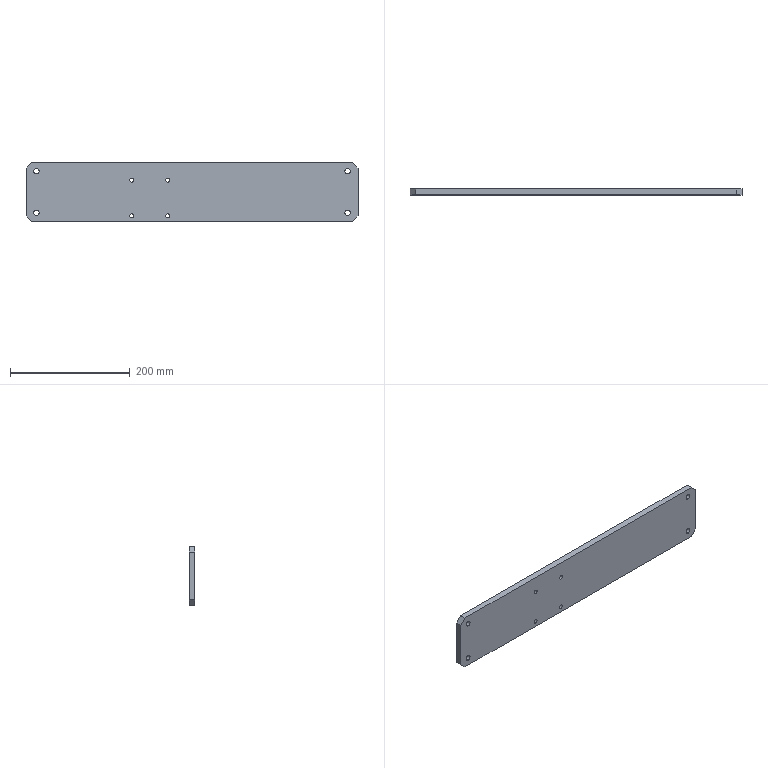Part | NX | features BREP 1 | 1 solid | 26 faces | box 555 x 10 x 100 mm | volume 549003 mm3 | cylinder 16 | plane 10 | commonest cylinder face diameters 6.8 x8 9 x8
STEP:
#1=CARTESIAN_POINT('',(-100.5,10.,16.6));
#2=VERTEX_POINT('',#1);
#3=CARTESIAN_POINT('',(-100.5,10.,23.4));
#4=VERTEX_POINT('',#3);
#5=CARTESIAN_POINT('',(-100.5,10.,20.));
#6=DIRECTION('',(0.,1.,0.));
#7=DIRECTION('',(0.,0.,1.));
#8=AXIS2_PLACEMENT_3D('',#5,#6,#7);
#9=CIRCLE('',#8,3.4);
#10=EDGE_CURVE('',#2,#4,#9,.T.);
#11=ORIENTED_EDGE('',*,*,#10,.T.);
#12=CARTESIAN_POINT('',(-100.5,0.,23.4));
#13=VERTEX_POINT('',#12);
#14=CARTESIAN_POINT('',(-100.5,0.,23.4));
#15=DIRECTION('',(0.,-1.,0.));
#16=VECTOR('',#15,1000.);
#17=LINE('',#14,#16);
#18=EDGE_CURVE('',#4,#13,#17,.T.);
#19=ORIENTED_EDGE('',*,*,#18,.T.);
#20=CARTESIAN_POINT('',(-100.5,0.,16.6));
#21=VERTEX_POINT('',#20);
#22=CARTESIAN_POINT('',(-100.5,0.,20.));
#23=DIRECTION('',(0.,-1.,0.));
#24=DIRECTION('',(0.,0.,-1.));
#25=AXIS2_PLACEMENT_3D('',#22,#23,#24);
#26=CIRCLE('',#25,3.4);
#27=EDGE_CURVE('',#13,#21,#26,.T.);
#28=ORIENTED_EDGE('',*,*,#27,.T.);
#29=CARTESIAN_POINT('',(-100.5,0.,16.6));
#30=DIRECTION('',(0.,-1.,0.));
#31=VECTOR('',#30,1000.);
#32=LINE('',#29,#31);
#33=EDGE_CURVE('',#2,#21,#32,.T.);
#34=ORIENTED_EDGE('',*,*,#33,.F.);
#35=EDGE_LOOP('',(#11,#19,#28,#34));
#36=FACE_BOUND('',#35,.T.);
#37=CARTESIAN_POINT('',(-100.5,0.,20.));
#38=DIRECTION('',(0.,-1.,0.));
#39=DIRECTION('',(0.,0.,-1.));
#40=AXIS2_PLACEMENT_3D('',#37,#38,#39);
#41=CYLINDRICAL_SURFACE('',#40,3.4);
#42=ADVANCED_FACE('',(#36),#41,.F.);
#43=CARTESIAN_POINT('',(-40.5,10.,16.6));
#44=VERTEX_POINT('',#43);
#45=CARTESIAN_POINT('',(-40.5,10.,23.4));
#46=VERTEX_POINT('',#45);
#47=CARTESIAN_POINT('',(-40.5,10.,20.));
#48=DIRECTION('',(0.,1.,0.));
#49=DIRECTION('',(0.,0.,1.));
#50=AXIS2_PLACEMENT_3D('',#47,#48,#49);
#51=CIRCLE('',#50,3.4);
#52=EDGE_CURVE('',#44,#46,#51,.T.);
#53=ORIENTED_EDGE('',*,*,#52,.T.);
#54=CARTESIAN_POINT('',(-40.5,0.,23.4));
#55=VERTEX_POINT('',#54);
#56=CARTESIAN_POINT('',(-40.5,0.,23.4));
#57=DIRECTION('',(0.,-1.,0.));
#58=VECTOR('',#57,1000.);
#59=LINE('',#56,#58);
#60=EDGE_CURVE('',#46,#55,#59,.T.);
#61=ORIENTED_EDGE('',*,*,#60,.T.);
#62=CARTESIAN_POINT('',(-40.5,0.,16.6));
#63=VERTEX_POINT('',#62);
#64=CARTESIAN_POINT('',(-40.5,0.,20.));
#65=DIRECTION('',(0.,-1.,0.));
#66=DIRECTION('',(0.,0.,-1.));
#67=AXIS2_PLACEMENT_3D('',#64,#65,#66);
#68=CIRCLE('',#67,3.4);
#69=EDGE_CURVE('',#55,#63,#68,.T.);
#70=ORIENTED_EDGE('',*,*,#69,.T.);
#71=CARTESIAN_POINT('',(-40.5,0.,16.6));
#72=DIRECTION('',(0.,-1.,0.));
#73=VECTOR('',#72,1000.);
#74=LINE('',#71,#73);
#75=EDGE_CURVE('',#44,#63,#74,.T.);
#76=ORIENTED_EDGE('',*,*,#75,.F.);
#77=EDGE_LOOP('',(#53,#61,#70,#76));
#78=FACE_BOUND('',#77,.T.);
#79=CARTESIAN_POINT('',(-40.5,0.,20.));
#80=DIRECTION('',(0.,-1.,0.));
#81=DIRECTION('',(0.,0.,-1.));
#82=AXIS2_PLACEMENT_3D('',#79,#80,#81);
#83=CYLINDRICAL_SURFACE('',#82,3.4);
#84=ADVANCED_FACE('',(#78),#83,.F.);
#85=CARTESIAN_POINT('',(-40.5,10.,-43.4));
#86=VERTEX_POINT('',#85);
#87=CARTESIAN_POINT('',(-40.5,10.,-36.6));
#88=VERTEX_POINT('',#87);
#89=CARTESIAN_POINT('',(-40.5,10.,-40.));
#90=DIRECTION('',(0.,1.,0.));
#91=DIRECTION('',(0.,0.,1.));
#92=AXIS2_PLACEMENT_3D('',#89,#90,#91);
#93=CIRCLE('',#92,3.4);
#94=EDGE_CURVE('',#86,#88,#93,.T.);
#95=ORIENTED_EDGE('',*,*,#94,.T.);
#96=CARTESIAN_POINT('',(-40.5,0.,-36.6));
#97=VERTEX_POINT('',#96);
#98=CARTESIAN_POINT('',(-40.5,0.,-36.6));
#99=DIRECTION('',(0.,-1.,0.));
#100=VECTOR('',#99,1000.);
#101=LINE('',#98,#100);
#102=EDGE_CURVE('',#88,#97,#101,.T.);
#103=ORIENTED_EDGE('',*,*,#102,.T.);
#104=CARTESIAN_POINT('',(-40.5,0.,-43.4));
#105=VERTEX_POINT('',#104);
#106=CARTESIAN_POINT('',(-40.5,0.,-40.));
#107=DIRECTION('',(0.,-1.,0.));
#108=DIRECTION('',(0.,0.,-1.));
#109=AXIS2_PLACEMENT_3D('',#106,#107,#108);
#110=CIRCLE('',#109,3.4);
#111=EDGE_CURVE('',#97,#105,#110,.T.);
#112=ORIENTED_EDGE('',*,*,#111,.T.);
#113=CARTESIAN_POINT('',(-40.5,0.,-43.4));
#114=DIRECTION('',(0.,-1.,0.));
#115=VECTOR('',#114,1000.);
#116=LINE('',#113,#115);
#117=EDGE_CURVE('',#86,#105,#116,.T.);
#118=ORIENTED_EDGE('',*,*,#117,.F.);
#119=EDGE_LOOP('',(#95,#103,#112,#118));
#120=FACE_BOUND('',#119,.T.);
#121=CARTESIAN_POINT('',(-40.5,0.,-40.));
#122=DIRECTION('',(0.,-1.,0.));
#123=DIRECTION('',(0.,0.,-1.));
#124=AXIS2_PLACEMENT_3D('',#121,#122,#123);
#125=CYLINDRICAL_SURFACE('',#124,3.4);
#126=ADVANCED_FACE('',(#120),#125,.F.);
#127=CARTESIAN_POINT('',(-100.5,10.,-43.4));
#128=VERTEX_POINT('',#127);
#129=CARTESIAN_POINT('',(-100.5,10.,-36.6));
#130=VERTEX_POINT('',#129);
#131=CARTESIAN_POINT('',(-100.5,10.,-40.));
#132=DIRECTION('',(0.,1.,0.));
#133=DIRECTION('',(0.,0.,1.));
#134=AXIS2_PLACEMENT_3D('',#131,#132,#133);
#135=CIRCLE('',#134,3.4);
#136=EDGE_CURVE('',#128,#130,#135,.T.);
#137=ORIENTED_EDGE('',*,*,#136,.T.);
#138=CARTESIAN_POINT('',(-100.5,0.,-36.6));
#139=VERTEX_POINT('',#138);
#140=CARTESIAN_POINT('',(-100.5,0.,-36.6));
#141=DIRECTION('',(0.,-1.,0.));
#142=VECTOR('',#141,1000.);
#143=LINE('',#140,#142);
#144=EDGE_CURVE('',#130,#139,#143,.T.);
#145=ORIENTED_EDGE('',*,*,#144,.T.);
#146=CARTESIAN_POINT('',(-100.5,0.,-43.4));
#147=VERTEX_POINT('',#146);
#148=CARTESIAN_POINT('',(-100.5,0.,-40.));
#149=DIRECTION('',(0.,-1.,0.));
#150=DIRECTION('',(0.,0.,-1.));
#151=AXIS2_PLACEMENT_3D('',#148,#149,#150);
#152=CIRCLE('',#151,3.4);
#153=EDGE_CURVE('',#139,#147,#152,.T.);
#154=ORIENTED_EDGE('',*,*,#153,.T.);
#155=CARTESIAN_POINT('',(-100.5,0.,-43.4));
#156=DIRECTION('',(0.,-1.,0.));
#157=VECTOR('',#156,1000.);
#158=LINE('',#155,#157);
#159=EDGE_CURVE('',#128,#147,#158,.T.);
#160=ORIENTED_EDGE('',*,*,#159,.F.);
#161=EDGE_LOOP('',(#137,#145,#154,#160));
#162=FACE_BOUND('',#161,.T.);
#163=CARTESIAN_POINT('',(-100.5,0.,-40.));
#164=DIRECTION('',(0.,-1.,0.));
#165=DIRECTION('',(0.,0.,-1.));
#166=AXIS2_PLACEMENT_3D('',#163,#164,#165);
#167=CYLINDRICAL_SURFACE('',#166,3.4);
#168=ADVANCED_FACE('',(#162),#167,.F.);
#169=CARTESIAN_POINT('',(-260.,0.,-39.5));
#170=VERTEX_POINT('',#169);
#171=CARTESIAN_POINT('',(-260.,0.,-30.5));
#172=VERTEX_POINT('',#171);
#173=CARTESIAN_POINT('',(-260.,0.,-35.));
#174=DIRECTION('',(0.,1.,0.));
#175=DIRECTION('',(0.,0.,1.));
#176=AXIS2_PLACEMENT_3D('',#173,#174,#175);
#177=CIRCLE('',#176,4.5);
#178=EDGE_CURVE('',#170,#172,#177,.T.);
#179=ORIENTED_EDGE('',*,*,#178,.F.);
#180=CARTESIAN_POINT('',(-260.,10.,-39.5));
#181=VERTEX_POINT('',#180);
#182=CARTESIAN_POINT('',(-260.,10.,-39.5));
#183=DIRECTION('',(0.,1.,0.));
#184=VECTOR('',#183,1000.);
#185=LINE('',#182,#184);
#186=EDGE_CURVE('',#181,#170,#185,.F.);
#187=ORIENTED_EDGE('',*,*,#186,.F.);
#188=CARTESIAN_POINT('',(-260.,10.,-30.5));
#189=VERTEX_POINT('',#188);
#190=CARTESIAN_POINT('',(-260.,10.,-35.));
#191=DIRECTION('',(0.,1.,0.));
#192=DIRECTION('',(0.,0.,1.));
#193=AXIS2_PLACEMENT_3D('',#190,#191,#192);
#194=CIRCLE('',#193,4.5);
#195=EDGE_CURVE('',#181,#189,#194,.T.);
#196=ORIENTED_EDGE('',*,*,#195,.T.);
#197=CARTESIAN_POINT('',(-260.,10.,-30.5));
#198=DIRECTION('',(0.,1.,0.));
#199=VECTOR('',#198,1000.);
#200=LINE('',#197,#199);
#201=EDGE_CURVE('',#189,#172,#200,.F.);
#202=ORIENTED_EDGE('',*,*,#201,.T.);
#203=EDGE_LOOP('',(#179,#187,#196,#202));
#204=FACE_BOUND('',#203,.T.);
#205=CARTESIAN_POINT('',(-260.,10.,-35.));
#206=DIRECTION('',(0.,1.,0.));
#207=DIRECTION('',(0.,0.,1.));
#208=AXIS2_PLACEMENT_3D('',#205,#206,#207);
#209=CYLINDRICAL_SURFACE('',#208,4.5);
#210=ADVANCED_FACE('',(#204),#209,.F.);
#211=CARTESIAN_POINT('',(-260.,0.,30.5));
#212=VERTEX_POINT('',#211);
#213=CARTESIAN_POINT('',(-260.,0.,39.5));
#214=VERTEX_POINT('',#213);
#215=CARTESIAN_POINT('',(-260.,0.,35.));
#216=DIRECTION('',(0.,1.,0.));
#217=DIRECTION('',(0.,0.,1.));
#218=AXIS2_PLACEMENT_3D('',#215,#216,#217);
#219=CIRCLE('',#218,4.5);
#220=EDGE_CURVE('',#212,#214,#219,.T.);
#221=ORIENTED_EDGE('',*,*,#220,.F.);
#222=CARTESIAN_POINT('',(-260.,10.,30.5));
#223=VERTEX_POINT('',#222);
#224=CARTESIAN_POINT('',(-260.,10.,30.5));
#225=DIRECTION('',(0.,1.,0.));
#226=VECTOR('',#225,1000.);
#227=LINE('',#224,#226);
#228=EDGE_CURVE('',#223,#212,#227,.F.);
#229=ORIENTED_EDGE('',*,*,#228,.F.);
#230=CARTESIAN_POINT('',(-260.,10.,39.5));
#231=VERTEX_POINT('',#230);
#232=CARTESIAN_POINT('',(-260.,10.,35.));
#233=DIRECTION('',(0.,1.,0.));
#234=DIRECTION('',(0.,0.,1.));
#235=AXIS2_PLACEMENT_3D('',#232,#233,#234);
#236=CIRCLE('',#235,4.5);
#237=EDGE_CURVE('',#223,#231,#236,.T.);
#238=ORIENTED_EDGE('',*,*,#237,.T.);
#239=CARTESIAN_POINT('',(-260.,10.,39.5));
#240=DIRECTION('',(0.,1.,0.));
#241=VECTOR('',#240,1000.);
#242=LINE('',#239,#241);
#243=EDGE_CURVE('',#231,#214,#242,.F.);
#244=ORIENTED_EDGE('',*,*,#243,.T.);
#245=EDGE_LOOP('',(#221,#229,#238,#244));
#246=FACE_BOUND('',#245,.T.);
#247=CARTESIAN_POINT('',(-260.,10.,35.));
#248=DIRECTION('',(0.,1.,0.));
#249=DIRECTION('',(0.,0.,1.));
#250=AXIS2_PLACEMENT_3D('',#247,#248,#249);
#251=CYLINDRICAL_SURFACE('',#250,4.5);
#252=ADVANCED_FACE('',(#246),#251,.F.);
#253=CARTESIAN_POINT('',(260.,0.,-39.5));
#254=VERTEX_POINT('',#253);
#255=CARTESIAN_POINT('',(260.,0.,-30.5));
#256=VERTEX_POINT('',#255);
#257=CARTESIAN_POINT('',(260.,0.,-35.));
#258=DIRECTION('',(0.,1.,0.));
#259=DIRECTION('',(0.,0.,1.));
#260=AXIS2_PLACEMENT_3D('',#257,#258,#259);
#261=CIRCLE('',#260,4.5);
#262=EDGE_CURVE('',#254,#256,#261,.T.);
#263=ORIENTED_EDGE('',*,*,#262,.F.);
#264=CARTESIAN_POINT('',(260.,10.,-39.5));
#265=VERTEX_POINT('',#264);
#266=CARTESIAN_POINT('',(260.,10.,-39.5));
#267=DIRECTION('',(0.,1.,0.));
#268=VECTOR('',#267,1000.);
#269=LINE('',#266,#268);
#270=EDGE_CURVE('',#265,#254,#269,.F.);
#271=ORIENTED_EDGE('',*,*,#270,.F.);
#272=CARTESIAN_POINT('',(260.,10.,-30.5));
#273=VERTEX_POINT('',#272);
#274=CARTESIAN_POINT('',(260.,10.,-35.));
#275=DIRECTION('',(0.,1.,0.));
#276=DIRECTION('',(0.,0.,1.));
#277=AXIS2_PLACEMENT_3D('',#274,#275,#276);
#278=CIRCLE('',#277,4.5);
#279=EDGE_CURVE('',#265,#273,#278,.T.);
#280=ORIENTED_EDGE('',*,*,#279,.T.);
#281=CARTESIAN_POINT('',(260.,10.,-30.5));
#282=DIRECTION('',(0.,1.,0.));
#283=VECTOR('',#282,1000.);
#284=LINE('',#281,#283);
#285=EDGE_CURVE('',#273,#256,#284,.F.);
#286=ORIENTED_EDGE('',*,*,#285,.T.);
#287=EDGE_LOOP('',(#263,#271,#280,#286));
#288=FACE_BOUND('',#287,.T.);
#289=CARTESIAN_POINT('',(260.,10.,-35.));
#290=DIRECTION('',(0.,1.,0.));
#291=DIRECTION('',(0.,0.,1.));
#292=AXIS2_PLACEMENT_3D('',#289,#290,#291);
#293=CYLINDRICAL_SURFACE('',#292,4.5);
#294=ADVANCED_FACE('',(#288),#293,.F.);
#295=CARTESIAN_POINT('',(260.,0.,30.5));
#296=VERTEX_POINT('',#295);
#297=CARTESIAN_POINT('',(260.,0.,39.5));
#298=VERTEX_POINT('',#297);
#299=CARTESIAN_POINT('',(260.,0.,35.));
#300=DIRECTION('',(0.,1.,0.));
#301=DIRECTION('',(0.,0.,1.));
#302=AXIS2_PLACEMENT_3D('',#299,#300,#301);
#303=CIRCLE('',#302,4.5);
#304=EDGE_CURVE('',#296,#298,#303,.T.);
#305=ORIENTED_EDGE('',*,*,#304,.F.);
#306=CARTESIAN_POINT('',(260.,10.,30.5));
#307=VERTEX_POINT('',#306);
#308=CARTESIAN_POINT('',(260.,10.,30.5));
#309=DIRECTION('',(0.,1.,0.));
#310=VECTOR('',#309,1000.);
#311=LINE('',#308,#310);
#312=EDGE_CURVE('',#307,#296,#311,.F.);
#313=ORIENTED_EDGE('',*,*,#312,.F.);
#314=CARTESIAN_POINT('',(260.,10.,39.5));
#315=VERTEX_POINT('',#314);
#316=CARTESIAN_POINT('',(260.,10.,35.));
#317=DIRECTION('',(0.,1.,0.));
#318=DIRECTION('',(0.,0.,1.));
#319=AXIS2_PLACEMENT_3D('',#316,#317,#318);
#320=CIRCLE('',#319,4.5);
#321=EDGE_CURVE('',#307,#315,#320,.T.);
#322=ORIENTED_EDGE('',*,*,#321,.T.);
#323=CARTESIAN_POINT('',(260.,10.,39.5));
#324=DIRECTION('',(0.,1.,0.));
#325=VECTOR('',#324,1000.);
#326=LINE('',#323,#325);
#327=EDGE_CURVE('',#315,#298,#326,.F.);
#328=ORIENTED_EDGE('',*,*,#327,.T.);
#329=EDGE_LOOP('',(#305,#313,#322,#328));
#330=FACE_BOUND('',#329,.T.);
#331=CARTESIAN_POINT('',(260.,10.,35.));
#332=DIRECTION('',(0.,1.,0.));
#333=DIRECTION('',(0.,0.,1.));
#334=AXIS2_PLACEMENT_3D('',#331,#332,#333);
#335=CYLINDRICAL_SURFACE('',#334,4.5);
#336=ADVANCED_FACE('',(#330),#335,.F.);
#337=CARTESIAN_POINT('',(277.5,10.,40.));
#338=VERTEX_POINT('',#337);
#339=CARTESIAN_POINT('',(277.5,10.,-40.));
#340=VERTEX_POINT('',#339);
#341=CARTESIAN_POINT('',(277.5,10.,-50.));
#342=DIRECTION('',(0.,0.,-1.));
#343=VECTOR('',#342,1000.);
#344=LINE('',#341,#343);
#345=EDGE_CURVE('',#338,#340,#344,.T.);
#346=ORIENTED_EDGE('',*,*,#345,.F.);
#347=CARTESIAN_POINT('',(277.5,0.,40.));
#348=VERTEX_POINT('',#347);
#349=CARTESIAN_POINT('',(277.5,10.,40.));
#350=DIRECTION('',(0.,-1.,0.));
#351=VECTOR('',#350,1000.);
#352=LINE('',#349,#351);
#353=EDGE_CURVE('',#338,#348,#352,.T.);
#354=ORIENTED_EDGE('',*,*,#353,.T.);
#355=CARTESIAN_POINT('',(277.5,0.,-40.));
#356=VERTEX_POINT('',#355);
#357=CARTESIAN_POINT('',(277.5,0.,-50.));
#358=DIRECTION('',(0.,0.,-1.));
#359=VECTOR('',#358,1000.);
#360=LINE('',#357,#359);
#361=EDGE_CURVE('',#348,#356,#360,.T.);
#362=ORIENTED_EDGE('',*,*,#361,.T.);
#363=CARTESIAN_POINT('',(277.5,10.,-40.));
#364=DIRECTION('',(0.,1.,0.));
#365=VECTOR('',#364,1000.);
#366=LINE('',#363,#365);
#367=EDGE_CURVE('',#356,#340,#366,.T.);
#368=ORIENTED_EDGE('',*,*,#367,.T.);
#369=EDGE_LOOP('',(#346,#354,#362,#368));
#370=FACE_BOUND('',#369,.T.);
#371=CARTESIAN_POINT('',(277.5,10.,-50.));
#372=DIRECTION('',(-1.,0.,0.));
#373=DIRECTION('',(0.,1.,0.));
#374=AXIS2_PLACEMENT_3D('',#371,#372,#373);
#375=PLANE('',#374);
#376=ADVANCED_FACE('',(#370),#375,.F.);
#377=CARTESIAN_POINT('',(267.5,10.,-50.));
#378=VERTEX_POINT('',#377);
#379=CARTESIAN_POINT('',(-267.5,10.,-50.));
#380=VERTEX_POINT('',#379);
#381=CARTESIAN_POINT('',(-277.5,10.,-50.));
#382=DIRECTION('',(-1.,0.,0.));
#383=VECTOR('',#382,1000.);
#384=LINE('',#381,#383);
#385=EDGE_CURVE('',#378,#380,#384,.T.);
#386=ORIENTED_EDGE('',*,*,#385,.F.);
#387=CARTESIAN_POINT('',(267.5,0.,-50.));
#388=VERTEX_POINT('',#387);
#389=CARTESIAN_POINT('',(267.5,10.,-50.));
#390=DIRECTION('',(0.,-1.,0.));
#391=VECTOR('',#390,1000.);
#392=LINE('',#389,#391);
#393=EDGE_CURVE('',#378,#388,#392,.T.);
#394=ORIENTED_EDGE('',*,*,#393,.T.);
#395=CARTESIAN_POINT('',(-267.5,0.,-50.));
#396=VERTEX_POINT('',#395);
#397=CARTESIAN_POINT('',(-277.5,0.,-50.));
#398=DIRECTION('',(-1.,0.,0.));
#399=VECTOR('',#398,1000.);
#400=LINE('',#397,#399);
#401=EDGE_CURVE('',#388,#396,#400,.T.);
#402=ORIENTED_EDGE('',*,*,#401,.T.);
#403=CARTESIAN_POINT('',(-267.5,10.,-50.));
#404=DIRECTION('',(0.,1.,0.));
#405=VECTOR('',#404,1000.);
#406=LINE('',#403,#405);
#407=EDGE_CURVE('',#396,#380,#406,.T.);
#408=ORIENTED_EDGE('',*,*,#407,.T.);
#409=EDGE_LOOP('',(#386,#394,#402,#408));
#410=FACE_BOUND('',#409,.T.);
#411=CARTESIAN_POINT('',(-277.5,10.,-50.));
#412=DIRECTION('',(0.,0.,1.));
#413=DIRECTION('',(1.,0.,0.));
#414=AXIS2_PLACEMENT_3D('',#411,#412,#413);
#415=PLANE('',#414);
#416=ADVANCED_FACE('',(#410),#415,.F.);
#417=CARTESIAN_POINT('',(-277.5,0.,-40.));
#418=VERTEX_POINT('',#417);
#419=CARTESIAN_POINT('',(-277.5,0.,40.));
#420=VERTEX_POINT('',#419);
#421=CARTESIAN_POINT('',(-277.5,0.,-50.));
#422=DIRECTION('',(0.,0.,1.));
#423=VECTOR('',#422,1000.);
#424=LINE('',#421,#423);
#425=EDGE_CURVE('',#418,#420,#424,.T.);
#426=ORIENTED_EDGE('',*,*,#425,.T.);
#427=CARTESIAN_POINT('',(-277.5,10.,40.));
#428=VERTEX_POINT('',#427);
#429=CARTESIAN_POINT('',(-277.5,10.,40.));
#430=DIRECTION('',(0.,1.,0.));
#431=VECTOR('',#430,1000.);
#432=LINE('',#429,#431);
#433=EDGE_CURVE('',#420,#428,#432,.T.);
#434=ORIENTED_EDGE('',*,*,#433,.T.);
#435=CARTESIAN_POINT('',(-277.5,10.,-40.));
#436=VERTEX_POINT('',#435);
#437=CARTESIAN_POINT('',(-277.5,10.,-50.));
#438=DIRECTION('',(0.,0.,1.));
#439=VECTOR('',#438,1000.);
#440=LINE('',#437,#439);
#441=EDGE_CURVE('',#436,#428,#440,.T.);
#442=ORIENTED_EDGE('',*,*,#441,.F.);
#443=CARTESIAN_POINT('',(-277.5,10.,-40.));
#444=DIRECTION('',(0.,-1.,0.));
#445=VECTOR('',#444,1000.);
#446=LINE('',#443,#445);
#447=EDGE_CURVE('',#436,#418,#446,.T.);
#448=ORIENTED_EDGE('',*,*,#447,.T.);
#449=EDGE_LOOP('',(#426,#434,#442,#448));
#450=FACE_BOUND('',#449,.T.);
#451=CARTESIAN_POINT('',(-277.5,10.,-50.));
#452=DIRECTION('',(1.,0.,0.));
#453=DIRECTION('',(0.,0.,-1.));
#454=AXIS2_PLACEMENT_3D('',#451,#452,#453);
#455=PLANE('',#454);
#456=ADVANCED_FACE('',(#450),#455,.F.);
#457=CARTESIAN_POINT('',(-267.5,0.,50.));
#458=VERTEX_POINT('',#457);
#459=CARTESIAN_POINT('',(267.5,0.,50.));
#460=VERTEX_POINT('',#459);
#461=CARTESIAN_POINT('',(-277.5,0.,50.));
#462=DIRECTION('',(1.,0.,0.));
#463=VECTOR('',#462,1000.);
#464=LINE('',#461,#463);
#465=EDGE_CURVE('',#458,#460,#464,.T.);
#466=ORIENTED_EDGE('',*,*,#465,.T.);
#467=CARTESIAN_POINT('',(267.5,10.,50.));
#468=VERTEX_POINT('',#467);
#469=CARTESIAN_POINT('',(267.5,10.,50.));
#470=DIRECTION('',(0.,1.,0.));
#471=VECTOR('',#470,1000.);
#472=LINE('',#469,#471);
#473=EDGE_CURVE('',#460,#468,#472,.T.);
#474=ORIENTED_EDGE('',*,*,#473,.T.);
#475=CARTESIAN_POINT('',(-267.5,10.,50.));
#476=VERTEX_POINT('',#475);
#477=CARTESIAN_POINT('',(-277.5,10.,50.));
#478=DIRECTION('',(1.,0.,0.));
#479=VECTOR('',#478,1000.);
#480=LINE('',#477,#479);
#481=EDGE_CURVE('',#476,#468,#480,.T.);
#482=ORIENTED_EDGE('',*,*,#481,.F.);
#483=CARTESIAN_POINT('',(-267.5,10.,50.));
#484=DIRECTION('',(0.,-1.,0.));
#485=VECTOR('',#484,1000.);
#486=LINE('',#483,#485);
#487=EDGE_CURVE('',#476,#458,#486,.T.);
#488=ORIENTED_EDGE('',*,*,#487,.T.);
#489=EDGE_LOOP('',(#466,#474,#482,#488));
#490=FACE_BOUND('',#489,.T.);
#491=CARTESIAN_POINT('',(-277.5,10.,50.));
#492=DIRECTION('',(0.,0.,-1.));
#493=DIRECTION('',(0.,-1.,0.));
#494=AXIS2_PLACEMENT_3D('',#491,#492,#493);
#495=PLANE('',#494);
#496=ADVANCED_FACE('',(#490),#495,.F.);
#497=ORIENTED_EDGE('',*,*,#481,.T.);
#498=CARTESIAN_POINT('',(158.75,10.,158.75));
#499=DIRECTION('',(0.7071,0.,-0.7071));
#500=VECTOR('',#499,1000.);
#501=LINE('',#498,#500);
#502=EDGE_CURVE('',#468,#338,#501,.T.);
#503=ORIENTED_EDGE('',*,*,#502,.T.);
#504=ORIENTED_EDGE('',*,*,#345,.T.);
#505=CARTESIAN_POINT('',(158.75,10.,-158.75));
#506=DIRECTION('',(-0.7071,0.,-0.7071));
#507=VECTOR('',#506,1000.);
#508=LINE('',#505,#507);
#509=EDGE_CURVE('',#340,#378,#508,.T.);
#510=ORIENTED_EDGE('',*,*,#509,.T.);
#511=ORIENTED_EDGE('',*,*,#385,.T.);
#512=CARTESIAN_POINT('',(-158.75,10.,-158.75));
#513=DIRECTION('',(-0.7071,0.,0.7071));
#514=VECTOR('',#513,1000.);
#515=LINE('',#512,#514);
#516=EDGE_CURVE('',#380,#436,#515,.T.);
#517=ORIENTED_EDGE('',*,*,#516,.T.);
#518=ORIENTED_EDGE('',*,*,#441,.T.);
#519=CARTESIAN_POINT('',(-158.75,10.,158.75));
#520=DIRECTION('',(0.7071,0.,0.7071));
#521=VECTOR('',#520,1000.);
#522=LINE('',#519,#521);
#523=EDGE_CURVE('',#428,#476,#522,.T.);
#524=ORIENTED_EDGE('',*,*,#523,.T.);
#525=EDGE_LOOP('',(#497,#503,#504,#510,#511,#517,#518,#524));
#526=FACE_BOUND('',#525,.T.);
#527=ORIENTED_EDGE('',*,*,#10,.F.);
#528=CARTESIAN_POINT('',(-100.5,10.,20.));
#529=DIRECTION('',(0.,1.,0.));
#530=DIRECTION('',(0.,0.,1.));
#531=AXIS2_PLACEMENT_3D('',#528,#529,#530);
#532=CIRCLE('',#531,3.4);
#533=EDGE_CURVE('',#4,#2,#532,.T.);
#534=ORIENTED_EDGE('',*,*,#533,.F.);
#535=EDGE_LOOP('',(#527,#534));
#536=FACE_BOUND('',#535,.T.);
#537=ORIENTED_EDGE('',*,*,#52,.F.);
#538=CARTESIAN_POINT('',(-40.5,10.,20.));
#539=DIRECTION('',(0.,1.,0.));
#540=DIRECTION('',(0.,0.,1.));
#541=AXIS2_PLACEMENT_3D('',#538,#539,#540);
#542=CIRCLE('',#541,3.4);
#543=EDGE_CURVE('',#46,#44,#542,.T.);
#544=ORIENTED_EDGE('',*,*,#543,.F.);
#545=EDGE_LOOP('',(#537,#544));
#546=FACE_BOUND('',#545,.T.);
#547=ORIENTED_EDGE('',*,*,#94,.F.);
#548=CARTESIAN_POINT('',(-40.5,10.,-40.));
#549=DIRECTION('',(0.,1.,0.));
#550=DIRECTION('',(0.,0.,1.));
#551=AXIS2_PLACEMENT_3D('',#548,#549,#550);
#552=CIRCLE('',#551,3.4);
#553=EDGE_CURVE('',#88,#86,#552,.T.);
#554=ORIENTED_EDGE('',*,*,#553,.F.);
#555=EDGE_LOOP('',(#547,#554));
#556=FACE_BOUND('',#555,.T.);
#557=ORIENTED_EDGE('',*,*,#136,.F.);
#558=CARTESIAN_POINT('',(-100.5,10.,-40.));
#559=DIRECTION('',(0.,1.,0.));
#560=DIRECTION('',(0.,0.,1.));
#561=AXIS2_PLACEMENT_3D('',#558,#559,#560);
#562=CIRCLE('',#561,3.4);
#563=EDGE_CURVE('',#130,#128,#562,.T.);
#564=ORIENTED_EDGE('',*,*,#563,.F.);
#565=EDGE_LOOP('',(#557,#564));
#566=FACE_BOUND('',#565,.T.);
#567=CARTESIAN_POINT('',(-260.,10.,-35.));
#568=DIRECTION('',(0.,1.,0.));
#569=DIRECTION('',(0.,0.,1.));
#570=AXIS2_PLACEMENT_3D('',#567,#568,#569);
#571=CIRCLE('',#570,4.5);
#572=EDGE_CURVE('',#189,#181,#571,.T.);
#573=ORIENTED_EDGE('',*,*,#572,.F.);
#574=ORIENTED_EDGE('',*,*,#195,.F.);
#575=EDGE_LOOP('',(#573,#574));
#576=FACE_BOUND('',#575,.T.);
#577=CARTESIAN_POINT('',(-260.,10.,35.));
#578=DIRECTION('',(0.,1.,0.));
#579=DIRECTION('',(0.,0.,1.));
#580=AXIS2_PLACEMENT_3D('',#577,#578,#579);
#581=CIRCLE('',#580,4.5);
#582=EDGE_CURVE('',#231,#223,#581,.T.);
#583=ORIENTED_EDGE('',*,*,#582,.F.);
#584=ORIENTED_EDGE('',*,*,#237,.F.);
#585=EDGE_LOOP('',(#583,#584));
#586=FACE_BOUND('',#585,.T.);
#587=CARTESIAN_POINT('',(260.,10.,-35.));
#588=DIRECTION('',(0.,1.,0.));
#589=DIRECTION('',(0.,0.,1.));
#590=AXIS2_PLACEMENT_3D('',#587,#588,#589);
#591=CIRCLE('',#590,4.5);
#592=EDGE_CURVE('',#273,#265,#591,.T.);
#593=ORIENTED_EDGE('',*,*,#592,.F.);
#594=ORIENTED_EDGE('',*,*,#279,.F.);
#595=EDGE_LOOP('',(#593,#594));
#596=FACE_BOUND('',#595,.T.);
#597=CARTESIAN_POINT('',(260.,10.,35.));
#598=DIRECTION('',(0.,1.,0.));
#599=DIRECTION('',(0.,0.,1.));
#600=AXIS2_PLACEMENT_3D('',#597,#598,#599);
#601=CIRCLE('',#600,4.5);
#602=EDGE_CURVE('',#315,#307,#601,.T.);
#603=ORIENTED_EDGE('',*,*,#602,.F.);
#604=ORIENTED_EDGE('',*,*,#321,.F.);
#605=EDGE_LOOP('',(#603,#604));
#606=FACE_BOUND('',#605,.T.);
#607=CARTESIAN_POINT('',(0.,10.,0.));
#608=DIRECTION('',(0.,1.,0.));
#609=DIRECTION('',(1.,0.,0.));
#610=AXIS2_PLACEMENT_3D('',#607,#608,#609);
#611=PLANE('',#610);
#612=ADVANCED_FACE('',(#526,#536,#546,#556,#566,#576,#586,#596,#606),#611,.T.);
#613=ORIENTED_EDGE('',*,*,#361,.F.);
#614=CARTESIAN_POINT('',(277.5,0.,40.));
#615=DIRECTION('',(-0.7071,0.,0.7071));
#616=VECTOR('',#615,1000.);
#617=LINE('',#614,#616);
#618=EDGE_CURVE('',#348,#460,#617,.T.);
#619=ORIENTED_EDGE('',*,*,#618,.T.);
#620=ORIENTED_EDGE('',*,*,#465,.F.);
#621=CARTESIAN_POINT('',(-267.5,0.,50.));
#622=DIRECTION('',(-0.7071,0.,-0.7071));
#623=VECTOR('',#622,1000.);
#624=LINE('',#621,#623);
#625=EDGE_CURVE('',#458,#420,#624,.T.);
#626=ORIENTED_EDGE('',*,*,#625,.T.);
#627=ORIENTED_EDGE('',*,*,#425,.F.);
#628=CARTESIAN_POINT('',(-277.5,0.,-40.));
#629=DIRECTION('',(0.7071,0.,-0.7071));
#630=VECTOR('',#629,1000.);
#631=LINE('',#628,#630);
#632=EDGE_CURVE('',#418,#396,#631,.T.);
#633=ORIENTED_EDGE('',*,*,#632,.T.);
#634=ORIENTED_EDGE('',*,*,#401,.F.);
#635=CARTESIAN_POINT('',(267.5,0.,-50.));
#636=DIRECTION('',(0.7071,0.,0.7071));
#637=VECTOR('',#636,1000.);
#638=LINE('',#635,#637);
#639=EDGE_CURVE('',#388,#356,#638,.T.);
#640=ORIENTED_EDGE('',*,*,#639,.T.);
#641=EDGE_LOOP('',(#613,#619,#620,#626,#627,#633,#634,#640));
#642=FACE_BOUND('',#641,.T.);
#643=CARTESIAN_POINT('',(-100.5,0.,20.));
#644=DIRECTION('',(0.,-1.,0.));
#645=DIRECTION('',(0.,0.,-1.));
#646=AXIS2_PLACEMENT_3D('',#643,#644,#645);
#647=CIRCLE('',#646,3.4);
#648=EDGE_CURVE('',#21,#13,#647,.T.);
#649=ORIENTED_EDGE('',*,*,#648,.F.);
#650=ORIENTED_EDGE('',*,*,#27,.F.);
#651=EDGE_LOOP('',(#649,#650));
#652=FACE_BOUND('',#651,.T.);
#653=CARTESIAN_POINT('',(-40.5,0.,20.));
#654=DIRECTION('',(0.,-1.,0.));
#655=DIRECTION('',(0.,0.,-1.));
#656=AXIS2_PLACEMENT_3D('',#653,#654,#655);
#657=CIRCLE('',#656,3.4);
#658=EDGE_CURVE('',#63,#55,#657,.T.);
#659=ORIENTED_EDGE('',*,*,#658,.F.);
#660=ORIENTED_EDGE('',*,*,#69,.F.);
#661=EDGE_LOOP('',(#659,#660));
#662=FACE_BOUND('',#661,.T.);
#663=CARTESIAN_POINT('',(-40.5,0.,-40.));
#664=DIRECTION('',(0.,-1.,0.));
#665=DIRECTION('',(0.,0.,-1.));
#666=AXIS2_PLACEMENT_3D('',#663,#664,#665);
#667=CIRCLE('',#666,3.4);
#668=EDGE_CURVE('',#105,#97,#667,.T.);
#669=ORIENTED_EDGE('',*,*,#668,.F.);
#670=ORIENTED_EDGE('',*,*,#111,.F.);
#671=EDGE_LOOP('',(#669,#670));
#672=FACE_BOUND('',#671,.T.);
#673=CARTESIAN_POINT('',(-100.5,0.,-40.));
#674=DIRECTION('',(0.,-1.,0.));
#675=DIRECTION('',(0.,0.,-1.));
#676=AXIS2_PLACEMENT_3D('',#673,#674,#675);
#677=CIRCLE('',#676,3.4);
#678=EDGE_CURVE('',#147,#139,#677,.T.);
#679=ORIENTED_EDGE('',*,*,#678,.F.);
#680=ORIENTED_EDGE('',*,*,#153,.F.);
#681=EDGE_LOOP('',(#679,#680));
#682=FACE_BOUND('',#681,.T.);
#683=CARTESIAN_POINT('',(-260.,0.,-35.));
#684=DIRECTION('',(0.,1.,0.));
#685=DIRECTION('',(0.,0.,1.));
#686=AXIS2_PLACEMENT_3D('',#683,#684,#685);
#687=CIRCLE('',#686,4.5);
#688=EDGE_CURVE('',#172,#170,#687,.T.);
#689=ORIENTED_EDGE('',*,*,#688,.T.);
#690=ORIENTED_EDGE('',*,*,#178,.T.);
#691=EDGE_LOOP('',(#689,#690));
#692=FACE_BOUND('',#691,.T.);
#693=CARTESIAN_POINT('',(-260.,0.,35.));
#694=DIRECTION('',(0.,1.,0.));
#695=DIRECTION('',(0.,0.,1.));
#696=AXIS2_PLACEMENT_3D('',#693,#694,#695);
#697=CIRCLE('',#696,4.5);
#698=EDGE_CURVE('',#214,#212,#697,.T.);
#699=ORIENTED_EDGE('',*,*,#698,.T.);
#700=ORIENTED_EDGE('',*,*,#220,.T.);
#701=EDGE_LOOP('',(#699,#700));
#702=FACE_BOUND('',#701,.T.);
#703=CARTESIAN_POINT('',(260.,0.,-35.));
#704=DIRECTION('',(0.,1.,0.));
#705=DIRECTION('',(0.,0.,1.));
#706=AXIS2_PLACEMENT_3D('',#703,#704,#705);
#707=CIRCLE('',#706,4.5);
#708=EDGE_CURVE('',#256,#254,#707,.T.);
#709=ORIENTED_EDGE('',*,*,#708,.T.);
#710=ORIENTED_EDGE('',*,*,#262,.T.);
#711=EDGE_LOOP('',(#709,#710));
#712=FACE_BOUND('',#711,.T.);
#713=CARTESIAN_POINT('',(260.,0.,35.));
#714=DIRECTION('',(0.,1.,0.));
#715=DIRECTION('',(0.,0.,1.));
#716=AXIS2_PLACEMENT_3D('',#713,#714,#715);
#717=CIRCLE('',#716,4.5);
#718=EDGE_CURVE('',#298,#296,#717,.T.);
#719=ORIENTED_EDGE('',*,*,#718,.T.);
#720=ORIENTED_EDGE('',*,*,#304,.T.);
#721=EDGE_LOOP('',(#719,#720));
#722=FACE_BOUND('',#721,.T.);
#723=CARTESIAN_POINT('',(0.,0.,0.));
#724=DIRECTION('',(0.,1.,0.));
#725=DIRECTION('',(1.,0.,0.));
#726=AXIS2_PLACEMENT_3D('',#723,#724,#725);
#727=PLANE('',#726);
#728=ADVANCED_FACE('',(#642,#652,#662,#672,#682,#692,#702,#712,#722),#727,.F.);
#729=ORIENTED_EDGE('',*,*,#312,.T.);
#730=ORIENTED_EDGE('',*,*,#718,.F.);
#731=ORIENTED_EDGE('',*,*,#327,.F.);
#732=ORIENTED_EDGE('',*,*,#602,.T.);
#733=EDGE_LOOP('',(#729,#730,#731,#732));
#734=FACE_BOUND('',#733,.T.);
#735=CARTESIAN_POINT('',(260.,10.,35.));
#736=DIRECTION('',(0.,1.,0.));
#737=DIRECTION('',(0.,0.,1.));
#738=AXIS2_PLACEMENT_3D('',#735,#736,#737);
#739=CYLINDRICAL_SURFACE('',#738,4.5);
#740=ADVANCED_FACE('',(#734),#739,.F.);
#741=ORIENTED_EDGE('',*,*,#270,.T.);
#742=ORIENTED_EDGE('',*,*,#708,.F.);
#743=ORIENTED_EDGE('',*,*,#285,.F.);
#744=ORIENTED_EDGE('',*,*,#592,.T.);
#745=EDGE_LOOP('',(#741,#742,#743,#744));
#746=FACE_BOUND('',#745,.T.);
#747=CARTESIAN_POINT('',(260.,10.,-35.));
#748=DIRECTION('',(0.,1.,0.));
#749=DIRECTION('',(0.,0.,1.));
#750=AXIS2_PLACEMENT_3D('',#747,#748,#749);
#751=CYLINDRICAL_SURFACE('',#750,4.5);
#752=ADVANCED_FACE('',(#746),#751,.F.);
#753=ORIENTED_EDGE('',*,*,#228,.T.);
#754=ORIENTED_EDGE('',*,*,#698,.F.);
#755=ORIENTED_EDGE('',*,*,#243,.F.);
#756=ORIENTED_EDGE('',*,*,#582,.T.);
#757=EDGE_LOOP('',(#753,#754,#755,#756));
#758=FACE_BOUND('',#757,.T.);
#759=CARTESIAN_POINT('',(-260.,10.,35.));
#760=DIRECTION('',(0.,1.,0.));
#761=DIRECTION('',(0.,0.,1.));
#762=AXIS2_PLACEMENT_3D('',#759,#760,#761);
#763=CYLINDRICAL_SURFACE('',#762,4.5);
#764=ADVANCED_FACE('',(#758),#763,.F.);
#765=ORIENTED_EDGE('',*,*,#186,.T.);
#766=ORIENTED_EDGE('',*,*,#688,.F.);
#767=ORIENTED_EDGE('',*,*,#201,.F.);
#768=ORIENTED_EDGE('',*,*,#572,.T.);
#769=EDGE_LOOP('',(#765,#766,#767,#768));
#770=FACE_BOUND('',#769,.T.);
#771=CARTESIAN_POINT('',(-260.,10.,-35.));
#772=DIRECTION('',(0.,1.,0.));
#773=DIRECTION('',(0.,0.,1.));
#774=AXIS2_PLACEMENT_3D('',#771,#772,#773);
#775=CYLINDRICAL_SURFACE('',#774,4.5);
#776=ADVANCED_FACE('',(#770),#775,.F.);
#777=ORIENTED_EDGE('',*,*,#502,.F.);
#778=ORIENTED_EDGE('',*,*,#473,.F.);
#779=ORIENTED_EDGE('',*,*,#618,.F.);
#780=ORIENTED_EDGE('',*,*,#353,.F.);
#781=EDGE_LOOP('',(#777,#778,#779,#780));
#782=FACE_BOUND('',#781,.T.);
#783=CARTESIAN_POINT('',(277.5,10.,40.));
#784=DIRECTION('',(-0.7071,0.,-0.7071));
#785=DIRECTION('',(-0.7071,0.,0.7071));
#786=AXIS2_PLACEMENT_3D('',#783,#784,#785);
#787=PLANE('',#786);
#788=ADVANCED_FACE('',(#782),#787,.F.);
#789=ORIENTED_EDGE('',*,*,#509,.F.);
#790=ORIENTED_EDGE('',*,*,#367,.F.);
#791=ORIENTED_EDGE('',*,*,#639,.F.);
#792=ORIENTED_EDGE('',*,*,#393,.F.);
#793=EDGE_LOOP('',(#789,#790,#791,#792));
#794=FACE_BOUND('',#793,.T.);
#795=CARTESIAN_POINT('',(267.5,10.,-50.));
#796=DIRECTION('',(-0.7071,0.,0.7071));
#797=DIRECTION('',(0.,1.,0.));
#798=AXIS2_PLACEMENT_3D('',#795,#796,#797);
#799=PLANE('',#798);
#800=ADVANCED_FACE('',(#794),#799,.F.);
#801=ORIENTED_EDGE('',*,*,#523,.F.);
#802=ORIENTED_EDGE('',*,*,#433,.F.);
#803=ORIENTED_EDGE('',*,*,#625,.F.);
#804=ORIENTED_EDGE('',*,*,#487,.F.);
#805=EDGE_LOOP('',(#801,#802,#803,#804));
#806=FACE_BOUND('',#805,.T.);
#807=CARTESIAN_POINT('',(-267.5,10.,50.));
#808=DIRECTION('',(0.7071,0.,-0.7071));
#809=DIRECTION('',(0.,-1.,0.));
#810=AXIS2_PLACEMENT_3D('',#807,#808,#809);
#811=PLANE('',#810);
#812=ADVANCED_FACE('',(#806),#811,.F.);
#813=ORIENTED_EDGE('',*,*,#516,.F.);
#814=ORIENTED_EDGE('',*,*,#407,.F.);
#815=ORIENTED_EDGE('',*,*,#632,.F.);
#816=ORIENTED_EDGE('',*,*,#447,.F.);
#817=EDGE_LOOP('',(#813,#814,#815,#816));
#818=FACE_BOUND('',#817,.T.);
#819=CARTESIAN_POINT('',(-277.5,10.,-40.));
#820=DIRECTION('',(0.7071,0.,0.7071));
#821=DIRECTION('',(0.,-1.,0.));
#822=AXIS2_PLACEMENT_3D('',#819,#820,#821);
#823=PLANE('',#822);
#824=ADVANCED_FACE('',(#818),#823,.F.);
#825=ORIENTED_EDGE('',*,*,#144,.F.);
#826=ORIENTED_EDGE('',*,*,#563,.T.);
#827=ORIENTED_EDGE('',*,*,#159,.T.);
#828=ORIENTED_EDGE('',*,*,#678,.T.);
#829=EDGE_LOOP('',(#825,#826,#827,#828));
#830=FACE_BOUND('',#829,.T.);
#831=CARTESIAN_POINT('',(-100.5,0.,-40.));
#832=DIRECTION('',(0.,-1.,0.));
#833=DIRECTION('',(0.,0.,-1.));
#834=AXIS2_PLACEMENT_3D('',#831,#832,#833);
#835=CYLINDRICAL_SURFACE('',#834,3.4);
#836=ADVANCED_FACE('',(#830),#835,.F.);
#837=ORIENTED_EDGE('',*,*,#102,.F.);
#838=ORIENTED_EDGE('',*,*,#553,.T.);
#839=ORIENTED_EDGE('',*,*,#117,.T.);
#840=ORIENTED_EDGE('',*,*,#668,.T.);
#841=EDGE_LOOP('',(#837,#838,#839,#840));
#842=FACE_BOUND('',#841,.T.);
#843=CARTESIAN_POINT('',(-40.5,0.,-40.));
#844=DIRECTION('',(0.,-1.,0.));
#845=DIRECTION('',(0.,0.,-1.));
#846=AXIS2_PLACEMENT_3D('',#843,#844,#845);
#847=CYLINDRICAL_SURFACE('',#846,3.4);
#848=ADVANCED_FACE('',(#842),#847,.F.);
#849=ORIENTED_EDGE('',*,*,#60,.F.);
#850=ORIENTED_EDGE('',*,*,#543,.T.);
#851=ORIENTED_EDGE('',*,*,#75,.T.);
#852=ORIENTED_EDGE('',*,*,#658,.T.);
#853=EDGE_LOOP('',(#849,#850,#851,#852));
#854=FACE_BOUND('',#853,.T.);
#855=CARTESIAN_POINT('',(-40.5,0.,20.));
#856=DIRECTION('',(0.,-1.,0.));
#857=DIRECTION('',(0.,0.,-1.));
#858=AXIS2_PLACEMENT_3D('',#855,#856,#857);
#859=CYLINDRICAL_SURFACE('',#858,3.4);
#860=ADVANCED_FACE('',(#854),#859,.F.);
#861=ORIENTED_EDGE('',*,*,#18,.F.);
#862=ORIENTED_EDGE('',*,*,#533,.T.);
#863=ORIENTED_EDGE('',*,*,#33,.T.);
#864=ORIENTED_EDGE('',*,*,#648,.T.);
#865=EDGE_LOOP('',(#861,#862,#863,#864));
#866=FACE_BOUND('',#865,.T.);
#867=CARTESIAN_POINT('',(-100.5,0.,20.));
#868=DIRECTION('',(0.,-1.,0.));
#869=DIRECTION('',(0.,0.,-1.));
#870=AXIS2_PLACEMENT_3D('',#867,#868,#869);
#871=CYLINDRICAL_SURFACE('',#870,3.4);
#872=ADVANCED_FACE('',(#866),#871,.F.);
#873=CLOSED_SHELL('',(#42,#84,#126,#168,#210,#252,#294,#336,#376,#416,#456,#496,#612,#728,#740,#752,#764,#776,#788,#800,#812,#824,#836,#848,#860,#872));
#874=MANIFOLD_SOLID_BREP('',#873);
#875=(LENGTH_UNIT()NAMED_UNIT(*)SI_UNIT(.MILLI.,.METRE.));
#876=UNCERTAINTY_MEASURE_WITH_UNIT(LENGTH_MEASURE(0.00001),#875,'','');
#877=(NAMED_UNIT(*)PLANE_ANGLE_UNIT()SI_UNIT($,.RADIAN.));
#878=(NAMED_UNIT(*)SI_UNIT($,.STERADIAN.)SOLID_ANGLE_UNIT());
#879=(GEOMETRIC_REPRESENTATION_CONTEXT(3)GLOBAL_UNCERTAINTY_ASSIGNED_CONTEXT((#876))GLOBAL_UNIT_ASSIGNED_CONTEXT((#875,#877,#878))REPRESENTATION_CONTEXT('',''));
#880=ADVANCED_BREP_SHAPE_REPRESENTATION('',(#874),#879);